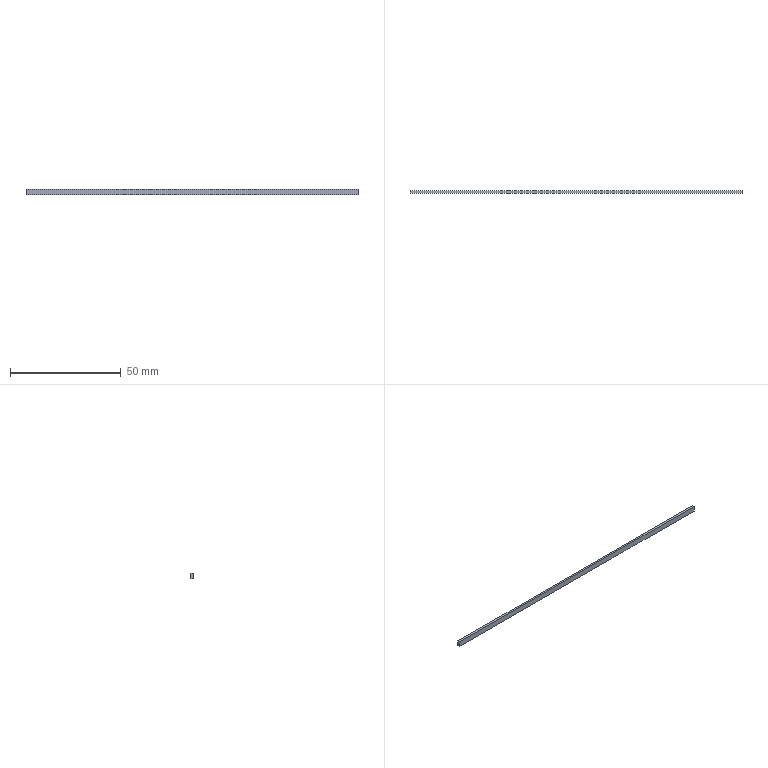Part | STEP file | TKR26H40-HS150 | 1 solid | 6 faces | box 150 x 1 x 2.6 mm | volume 390 mm3 | plane 6
STEP:
#1=CARTESIAN_POINT('',(0.,0.,0.));
#2=DIRECTION('',(0.,0.,1.));
#3=DIRECTION('',(1.,0.,0.));
#4=AXIS2_PLACEMENT_3D('',#1,#2,#3);
#5=CARTESIAN_POINT('',(50.,40.,0.));
#6=VERTEX_POINT('',#5);
#7=CARTESIAN_POINT('',(50.,39.,0.));
#8=VERTEX_POINT('',#7);
#9=CARTESIAN_POINT('',(50.,39.5,0.));
#10=DIRECTION('',(0.,-1.,0.));
#11=VECTOR('',#10,1.);
#12=LINE('',#9,#11);
#13=CARTESIAN_POINT('',(125.,39.5,0.));
#14=DIRECTION('',(0.,0.,-1.));
#15=DIRECTION('',(0.,1.,0.));
#16=AXIS2_PLACEMENT_3D('',#13,#14,#15);
#17=PLANE('',#16);
#18=CARTESIAN_POINT('',(0.,-75.));
#19=DIRECTION('',(-1.,0.));
#20=VECTOR('',#19,1.);
#21=LINE('',#18,#20);
#22=(GEOMETRIC_REPRESENTATION_CONTEXT(2)PARAMETRIC_REPRESENTATION_CONTEXT()REPRESENTATION_CONTEXT('',''));
#23=DEFINITIONAL_REPRESENTATION('',(#21),#22);
#24=PCURVE('',#17,#23);
#25=CARTESIAN_POINT('',(50.,39.5,2.6));
#26=DIRECTION('',(-1.,0.,0.));
#27=DIRECTION('',(0.,0.,1.));
#28=AXIS2_PLACEMENT_3D('',#25,#26,#27);
#29=PLANE('',#28);
#30=CARTESIAN_POINT('',(-2.6,0.));
#31=DIRECTION('',(0.,-1.));
#32=VECTOR('',#31,1.);
#33=LINE('',#30,#32);
#34=(GEOMETRIC_REPRESENTATION_CONTEXT(2)PARAMETRIC_REPRESENTATION_CONTEXT()REPRESENTATION_CONTEXT('',''));
#35=DEFINITIONAL_REPRESENTATION('',(#33),#34);
#36=PCURVE('',#29,#35);
#37=SURFACE_CURVE('',#12,(#24,#36),.PCURVE_S1.);
#38=EDGE_CURVE('',#6,#8,#37,.T.);
#39=ORIENTED_EDGE('',*,*,#38,.F.);
#40=CARTESIAN_POINT('',(200.,40.,0.));
#41=VERTEX_POINT('',#40);
#42=CARTESIAN_POINT('',(125.,40.,0.));
#43=DIRECTION('',(-1.,0.,0.));
#44=VECTOR('',#43,1.);
#45=LINE('',#42,#44);
#46=CARTESIAN_POINT('',(0.5,0.));
#47=DIRECTION('',(0.,-1.));
#48=VECTOR('',#47,1.);
#49=LINE('',#46,#48);
#50=(GEOMETRIC_REPRESENTATION_CONTEXT(2)PARAMETRIC_REPRESENTATION_CONTEXT()REPRESENTATION_CONTEXT('',''));
#51=DEFINITIONAL_REPRESENTATION('',(#49),#50);
#52=PCURVE('',#17,#51);
#53=CARTESIAN_POINT('',(125.,40.,2.6));
#54=DIRECTION('',(0.,1.,0.));
#55=DIRECTION('',(0.,0.,1.));
#56=AXIS2_PLACEMENT_3D('',#53,#54,#55);
#57=PLANE('',#56);
#58=CARTESIAN_POINT('',(-2.6,0.));
#59=DIRECTION('',(0.,-1.));
#60=VECTOR('',#59,1.);
#61=LINE('',#58,#60);
#62=(GEOMETRIC_REPRESENTATION_CONTEXT(2)PARAMETRIC_REPRESENTATION_CONTEXT()REPRESENTATION_CONTEXT('',''));
#63=DEFINITIONAL_REPRESENTATION('',(#61),#62);
#64=PCURVE('',#57,#63);
#65=SURFACE_CURVE('',#45,(#52,#64),.PCURVE_S1.);
#66=EDGE_CURVE('',#41,#6,#65,.T.);
#67=ORIENTED_EDGE('',*,*,#66,.F.);
#68=CARTESIAN_POINT('',(200.,39.,0.));
#69=VERTEX_POINT('',#68);
#70=CARTESIAN_POINT('',(200.,39.5,0.));
#71=DIRECTION('',(0.,1.,0.));
#72=VECTOR('',#71,1.);
#73=LINE('',#70,#72);
#74=CARTESIAN_POINT('',(0.,75.));
#75=DIRECTION('',(1.,0.));
#76=VECTOR('',#75,1.);
#77=LINE('',#74,#76);
#78=(GEOMETRIC_REPRESENTATION_CONTEXT(2)PARAMETRIC_REPRESENTATION_CONTEXT()REPRESENTATION_CONTEXT('',''));
#79=DEFINITIONAL_REPRESENTATION('',(#77),#78);
#80=PCURVE('',#17,#79);
#81=CARTESIAN_POINT('',(200.,39.5,2.6));
#82=DIRECTION('',(1.,0.,0.));
#83=DIRECTION('',(0.,0.,-1.));
#84=AXIS2_PLACEMENT_3D('',#81,#82,#83);
#85=PLANE('',#84);
#86=CARTESIAN_POINT('',(2.6,0.));
#87=DIRECTION('',(0.,1.));
#88=VECTOR('',#87,1.);
#89=LINE('',#86,#88);
#90=(GEOMETRIC_REPRESENTATION_CONTEXT(2)PARAMETRIC_REPRESENTATION_CONTEXT()REPRESENTATION_CONTEXT('',''));
#91=DEFINITIONAL_REPRESENTATION('',(#89),#90);
#92=PCURVE('',#85,#91);
#93=SURFACE_CURVE('',#73,(#80,#92),.PCURVE_S1.);
#94=EDGE_CURVE('',#69,#41,#93,.T.);
#95=ORIENTED_EDGE('',*,*,#94,.F.);
#96=CARTESIAN_POINT('',(125.,39.,0.));
#97=DIRECTION('',(1.,0.,0.));
#98=VECTOR('',#97,1.);
#99=LINE('',#96,#98);
#100=CARTESIAN_POINT('',(-0.5,0.));
#101=DIRECTION('',(0.,1.));
#102=VECTOR('',#101,1.);
#103=LINE('',#100,#102);
#104=(GEOMETRIC_REPRESENTATION_CONTEXT(2)PARAMETRIC_REPRESENTATION_CONTEXT()REPRESENTATION_CONTEXT('',''));
#105=DEFINITIONAL_REPRESENTATION('',(#103),#104);
#106=PCURVE('',#17,#105);
#107=CARTESIAN_POINT('',(125.,39.,2.6));
#108=DIRECTION('',(0.,-1.,0.));
#109=DIRECTION('',(0.,0.,-1.));
#110=AXIS2_PLACEMENT_3D('',#107,#108,#109);
#111=PLANE('',#110);
#112=CARTESIAN_POINT('',(2.6,0.));
#113=DIRECTION('',(0.,1.));
#114=VECTOR('',#113,1.);
#115=LINE('',#112,#114);
#116=(GEOMETRIC_REPRESENTATION_CONTEXT(2)PARAMETRIC_REPRESENTATION_CONTEXT()REPRESENTATION_CONTEXT('',''));
#117=DEFINITIONAL_REPRESENTATION('',(#115),#116);
#118=PCURVE('',#111,#117);
#119=SURFACE_CURVE('',#99,(#106,#118),.PCURVE_S1.);
#120=EDGE_CURVE('',#8,#69,#119,.T.);
#121=ORIENTED_EDGE('',*,*,#120,.F.);
#122=EDGE_LOOP('',(#39,#67,#95,#121));
#123=FACE_BOUND('',#122,.T.);
#124=ADVANCED_FACE('',(#123),#17,.T.);
#125=CARTESIAN_POINT('',(50.,40.,2.6));
#126=VERTEX_POINT('',#125);
#127=CARTESIAN_POINT('',(50.,40.,2.6));
#128=DIRECTION('',(0.,0.,-1.));
#129=VECTOR('',#128,1.);
#130=LINE('',#127,#129);
#131=CARTESIAN_POINT('',(0.,0.5));
#132=DIRECTION('',(-1.,0.));
#133=VECTOR('',#132,1.);
#134=LINE('',#131,#133);
#135=(GEOMETRIC_REPRESENTATION_CONTEXT(2)PARAMETRIC_REPRESENTATION_CONTEXT()REPRESENTATION_CONTEXT('',''));
#136=DEFINITIONAL_REPRESENTATION('',(#134),#135);
#137=PCURVE('',#29,#136);
#138=CARTESIAN_POINT('',(0.,-75.));
#139=DIRECTION('',(-1.,0.));
#140=VECTOR('',#139,1.);
#141=LINE('',#138,#140);
#142=(GEOMETRIC_REPRESENTATION_CONTEXT(2)PARAMETRIC_REPRESENTATION_CONTEXT()REPRESENTATION_CONTEXT('',''));
#143=DEFINITIONAL_REPRESENTATION('',(#141),#142);
#144=PCURVE('',#57,#143);
#145=SURFACE_CURVE('',#130,(#137,#144),.PCURVE_S1.);
#146=EDGE_CURVE('',#126,#6,#145,.T.);
#147=ORIENTED_EDGE('',*,*,#146,.T.);
#148=ORIENTED_EDGE('',*,*,#38,.T.);
#149=CARTESIAN_POINT('',(50.,39.,2.6));
#150=VERTEX_POINT('',#149);
#151=CARTESIAN_POINT('',(50.,39.,2.6));
#152=DIRECTION('',(0.,0.,-1.));
#153=VECTOR('',#152,1.);
#154=LINE('',#151,#153);
#155=CARTESIAN_POINT('',(0.,-0.5));
#156=DIRECTION('',(-1.,0.));
#157=VECTOR('',#156,1.);
#158=LINE('',#155,#157);
#159=(GEOMETRIC_REPRESENTATION_CONTEXT(2)PARAMETRIC_REPRESENTATION_CONTEXT()REPRESENTATION_CONTEXT('',''));
#160=DEFINITIONAL_REPRESENTATION('',(#158),#159);
#161=PCURVE('',#29,#160);
#162=CARTESIAN_POINT('',(0.,-75.));
#163=DIRECTION('',(1.,0.));
#164=VECTOR('',#163,1.);
#165=LINE('',#162,#164);
#166=(GEOMETRIC_REPRESENTATION_CONTEXT(2)PARAMETRIC_REPRESENTATION_CONTEXT()REPRESENTATION_CONTEXT('',''));
#167=DEFINITIONAL_REPRESENTATION('',(#165),#166);
#168=PCURVE('',#111,#167);
#169=SURFACE_CURVE('',#154,(#161,#168),.PCURVE_S1.);
#170=EDGE_CURVE('',#150,#8,#169,.T.);
#171=ORIENTED_EDGE('',*,*,#170,.F.);
#172=CARTESIAN_POINT('',(50.,39.5,2.6));
#173=DIRECTION('',(0.,1.,0.));
#174=VECTOR('',#173,1.);
#175=LINE('',#172,#174);
#176=CARTESIAN_POINT('',(0.,0.));
#177=DIRECTION('',(0.,1.));
#178=VECTOR('',#177,1.);
#179=LINE('',#176,#178);
#180=(GEOMETRIC_REPRESENTATION_CONTEXT(2)PARAMETRIC_REPRESENTATION_CONTEXT()REPRESENTATION_CONTEXT('',''));
#181=DEFINITIONAL_REPRESENTATION('',(#179),#180);
#182=PCURVE('',#29,#181);
#183=CARTESIAN_POINT('',(125.,39.5,2.6));
#184=DIRECTION('',(0.,0.,1.));
#185=DIRECTION('',(0.,-1.,0.));
#186=AXIS2_PLACEMENT_3D('',#183,#184,#185);
#187=PLANE('',#186);
#188=CARTESIAN_POINT('',(0.,-75.));
#189=DIRECTION('',(-1.,0.));
#190=VECTOR('',#189,1.);
#191=LINE('',#188,#190);
#192=(GEOMETRIC_REPRESENTATION_CONTEXT(2)PARAMETRIC_REPRESENTATION_CONTEXT()REPRESENTATION_CONTEXT('',''));
#193=DEFINITIONAL_REPRESENTATION('',(#191),#192);
#194=PCURVE('',#187,#193);
#195=SURFACE_CURVE('',#175,(#182,#194),.PCURVE_S1.);
#196=EDGE_CURVE('',#150,#126,#195,.T.);
#197=ORIENTED_EDGE('',*,*,#196,.T.);
#198=EDGE_LOOP('',(#147,#148,#171,#197));
#199=FACE_BOUND('',#198,.T.);
#200=ADVANCED_FACE('',(#199),#29,.T.);
#201=ORIENTED_EDGE('',*,*,#170,.T.);
#202=ORIENTED_EDGE('',*,*,#120,.T.);
#203=CARTESIAN_POINT('',(200.,39.,2.6));
#204=VERTEX_POINT('',#203);
#205=CARTESIAN_POINT('',(200.,39.,2.6));
#206=DIRECTION('',(0.,0.,-1.));
#207=VECTOR('',#206,1.);
#208=LINE('',#205,#207);
#209=CARTESIAN_POINT('',(0.,75.));
#210=DIRECTION('',(1.,0.));
#211=VECTOR('',#210,1.);
#212=LINE('',#209,#211);
#213=(GEOMETRIC_REPRESENTATION_CONTEXT(2)PARAMETRIC_REPRESENTATION_CONTEXT()REPRESENTATION_CONTEXT('',''));
#214=DEFINITIONAL_REPRESENTATION('',(#212),#213);
#215=PCURVE('',#111,#214);
#216=CARTESIAN_POINT('',(0.,-0.5));
#217=DIRECTION('',(1.,0.));
#218=VECTOR('',#217,1.);
#219=LINE('',#216,#218);
#220=(GEOMETRIC_REPRESENTATION_CONTEXT(2)PARAMETRIC_REPRESENTATION_CONTEXT()REPRESENTATION_CONTEXT('',''));
#221=DEFINITIONAL_REPRESENTATION('',(#219),#220);
#222=PCURVE('',#85,#221);
#223=SURFACE_CURVE('',#208,(#215,#222),.PCURVE_S1.);
#224=EDGE_CURVE('',#204,#69,#223,.T.);
#225=ORIENTED_EDGE('',*,*,#224,.F.);
#226=CARTESIAN_POINT('',(125.,39.,2.6));
#227=DIRECTION('',(-1.,0.,0.));
#228=VECTOR('',#227,1.);
#229=LINE('',#226,#228);
#230=CARTESIAN_POINT('',(0.,0.));
#231=DIRECTION('',(0.,-1.));
#232=VECTOR('',#231,1.);
#233=LINE('',#230,#232);
#234=(GEOMETRIC_REPRESENTATION_CONTEXT(2)PARAMETRIC_REPRESENTATION_CONTEXT()REPRESENTATION_CONTEXT('',''));
#235=DEFINITIONAL_REPRESENTATION('',(#233),#234);
#236=PCURVE('',#111,#235);
#237=CARTESIAN_POINT('',(0.5,0.));
#238=DIRECTION('',(0.,-1.));
#239=VECTOR('',#238,1.);
#240=LINE('',#237,#239);
#241=(GEOMETRIC_REPRESENTATION_CONTEXT(2)PARAMETRIC_REPRESENTATION_CONTEXT()REPRESENTATION_CONTEXT('',''));
#242=DEFINITIONAL_REPRESENTATION('',(#240),#241);
#243=PCURVE('',#187,#242);
#244=SURFACE_CURVE('',#229,(#236,#243),.PCURVE_S1.);
#245=EDGE_CURVE('',#204,#150,#244,.T.);
#246=ORIENTED_EDGE('',*,*,#245,.T.);
#247=EDGE_LOOP('',(#201,#202,#225,#246));
#248=FACE_BOUND('',#247,.T.);
#249=ADVANCED_FACE('',(#248),#111,.T.);
#250=ORIENTED_EDGE('',*,*,#224,.T.);
#251=ORIENTED_EDGE('',*,*,#94,.T.);
#252=CARTESIAN_POINT('',(200.,40.,2.6));
#253=VERTEX_POINT('',#252);
#254=CARTESIAN_POINT('',(200.,40.,2.6));
#255=DIRECTION('',(0.,0.,-1.));
#256=VECTOR('',#255,1.);
#257=LINE('',#254,#256);
#258=CARTESIAN_POINT('',(0.,0.5));
#259=DIRECTION('',(1.,0.));
#260=VECTOR('',#259,1.);
#261=LINE('',#258,#260);
#262=(GEOMETRIC_REPRESENTATION_CONTEXT(2)PARAMETRIC_REPRESENTATION_CONTEXT()REPRESENTATION_CONTEXT('',''));
#263=DEFINITIONAL_REPRESENTATION('',(#261),#262);
#264=PCURVE('',#85,#263);
#265=CARTESIAN_POINT('',(0.,75.));
#266=DIRECTION('',(-1.,0.));
#267=VECTOR('',#266,1.);
#268=LINE('',#265,#267);
#269=(GEOMETRIC_REPRESENTATION_CONTEXT(2)PARAMETRIC_REPRESENTATION_CONTEXT()REPRESENTATION_CONTEXT('',''));
#270=DEFINITIONAL_REPRESENTATION('',(#268),#269);
#271=PCURVE('',#57,#270);
#272=SURFACE_CURVE('',#257,(#264,#271),.PCURVE_S1.);
#273=EDGE_CURVE('',#253,#41,#272,.T.);
#274=ORIENTED_EDGE('',*,*,#273,.F.);
#275=CARTESIAN_POINT('',(200.,39.5,2.6));
#276=DIRECTION('',(0.,-1.,0.));
#277=VECTOR('',#276,1.);
#278=LINE('',#275,#277);
#279=CARTESIAN_POINT('',(0.,0.));
#280=DIRECTION('',(0.,-1.));
#281=VECTOR('',#280,1.);
#282=LINE('',#279,#281);
#283=(GEOMETRIC_REPRESENTATION_CONTEXT(2)PARAMETRIC_REPRESENTATION_CONTEXT()REPRESENTATION_CONTEXT('',''));
#284=DEFINITIONAL_REPRESENTATION('',(#282),#283);
#285=PCURVE('',#85,#284);
#286=CARTESIAN_POINT('',(0.,75.));
#287=DIRECTION('',(1.,0.));
#288=VECTOR('',#287,1.);
#289=LINE('',#286,#288);
#290=(GEOMETRIC_REPRESENTATION_CONTEXT(2)PARAMETRIC_REPRESENTATION_CONTEXT()REPRESENTATION_CONTEXT('',''));
#291=DEFINITIONAL_REPRESENTATION('',(#289),#290);
#292=PCURVE('',#187,#291);
#293=SURFACE_CURVE('',#278,(#285,#292),.PCURVE_S1.);
#294=EDGE_CURVE('',#253,#204,#293,.T.);
#295=ORIENTED_EDGE('',*,*,#294,.T.);
#296=EDGE_LOOP('',(#250,#251,#274,#295));
#297=FACE_BOUND('',#296,.T.);
#298=ADVANCED_FACE('',(#297),#85,.T.);
#299=CARTESIAN_POINT('',(125.,40.,2.6));
#300=DIRECTION('',(1.,0.,0.));
#301=VECTOR('',#300,1.);
#302=LINE('',#299,#301);
#303=CARTESIAN_POINT('',(-0.5,0.));
#304=DIRECTION('',(0.,1.));
#305=VECTOR('',#304,1.);
#306=LINE('',#303,#305);
#307=(GEOMETRIC_REPRESENTATION_CONTEXT(2)PARAMETRIC_REPRESENTATION_CONTEXT()REPRESENTATION_CONTEXT('',''));
#308=DEFINITIONAL_REPRESENTATION('',(#306),#307);
#309=PCURVE('',#187,#308);
#310=CARTESIAN_POINT('',(0.,0.));
#311=DIRECTION('',(0.,1.));
#312=VECTOR('',#311,1.);
#313=LINE('',#310,#312);
#314=(GEOMETRIC_REPRESENTATION_CONTEXT(2)PARAMETRIC_REPRESENTATION_CONTEXT()REPRESENTATION_CONTEXT('',''));
#315=DEFINITIONAL_REPRESENTATION('',(#313),#314);
#316=PCURVE('',#57,#315);
#317=SURFACE_CURVE('',#302,(#309,#316),.PCURVE_S1.);
#318=EDGE_CURVE('',#126,#253,#317,.T.);
#319=ORIENTED_EDGE('',*,*,#318,.F.);
#320=ORIENTED_EDGE('',*,*,#196,.F.);
#321=ORIENTED_EDGE('',*,*,#245,.F.);
#322=ORIENTED_EDGE('',*,*,#294,.F.);
#323=EDGE_LOOP('',(#319,#320,#321,#322));
#324=FACE_BOUND('',#323,.T.);
#325=ADVANCED_FACE('',(#324),#187,.T.);
#326=ORIENTED_EDGE('',*,*,#318,.T.);
#327=ORIENTED_EDGE('',*,*,#273,.T.);
#328=ORIENTED_EDGE('',*,*,#66,.T.);
#329=ORIENTED_EDGE('',*,*,#146,.F.);
#330=EDGE_LOOP('',(#326,#327,#328,#329));
#331=FACE_BOUND('',#330,.T.);
#332=ADVANCED_FACE('',(#331),#57,.T.);
#333=CLOSED_SHELL('',(#124,#200,#249,#298,#325,#332));
#334=MANIFOLD_SOLID_BREP('',#333);
#335=(LENGTH_UNIT()NAMED_UNIT(*)SI_UNIT(.MILLI.,.METRE.));
#336=UNCERTAINTY_MEASURE_WITH_UNIT(LENGTH_MEASURE(0.0000001),#335,'','');
#337=(NAMED_UNIT(*)PLANE_ANGLE_UNIT()SI_UNIT($,.RADIAN.));
#338=(NAMED_UNIT(*)SI_UNIT($,.STERADIAN.)SOLID_ANGLE_UNIT());
#339=(GEOMETRIC_REPRESENTATION_CONTEXT(3)GLOBAL_UNCERTAINTY_ASSIGNED_CONTEXT((#336))GLOBAL_UNIT_ASSIGNED_CONTEXT((#335,#337,#338))REPRESENTATION_CONTEXT('',''));
#340=ADVANCED_BREP_SHAPE_REPRESENTATION('',(#4,#334),#339);